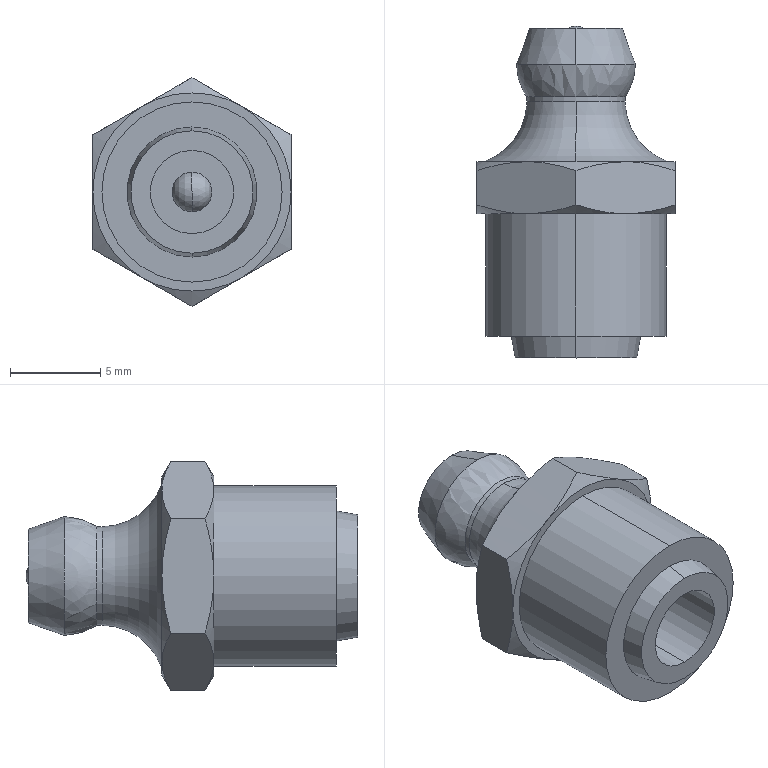Part | SolidWorks | features BaseBody 1 | 1 solid | 44 faces | box 11 x 18.425 x 12.702 mm | volume 861.691 mm3 | cone 17 | plane 12 | cylinder 6 | sphere 5 | torus 4 | commonest cylinder face diameters 2.21 x2 4.624 x2 10 x2